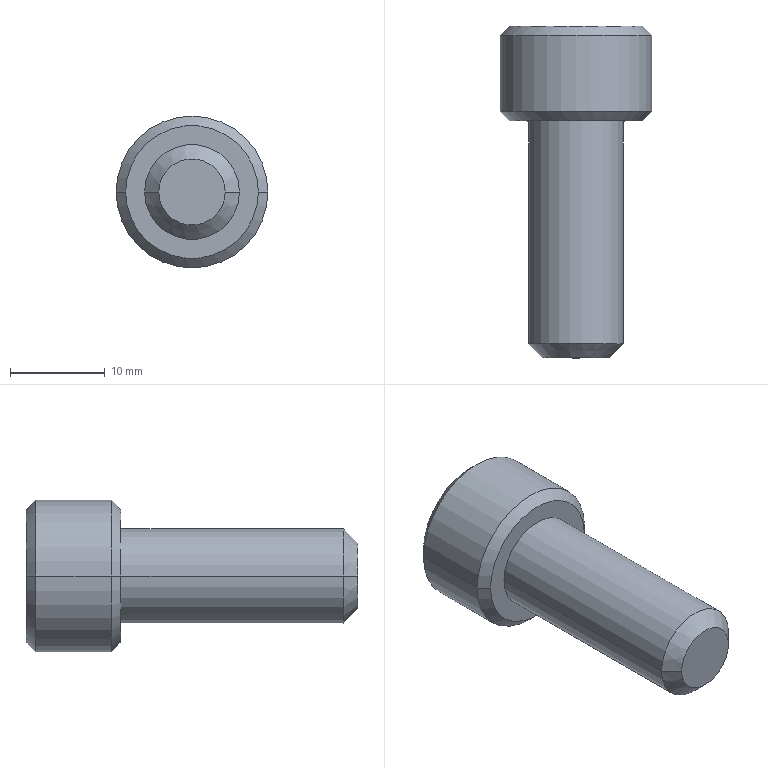Part | STEP file | BB62-M10-25L-1 | 1 solid | 27 faces | box 16 x 35 x 16 mm | volume 3564 mm3 | plane 15 | cone 8 | cylinder 4 | commonest cylinder face diameters 10 x2 16 x2
STEP:
#1=CARTESIAN_POINT('',(0.,2.359,0.));
#2=VERTEX_POINT('',#1);
#3=CARTESIAN_POINT('',(4.575,5.,0.));
#4=VERTEX_POINT('',#3);
#5=CARTESIAN_POINT('',(0.,2.359,0.));
#6=DIRECTION('',(0.866,0.5,0.));
#7=VECTOR('',#6,1000.);
#8=LINE('',#5,#7);
#9=EDGE_CURVE('',#2,#4,#8,.T.);
#10=ORIENTED_EDGE('',*,*,#9,.F.);
#11=CARTESIAN_POINT('',(-4.575,5.,0.));
#12=VERTEX_POINT('',#11);
#13=CARTESIAN_POINT('',(0.,2.359,0.));
#14=DIRECTION('',(-0.866,0.5,0.));
#15=VECTOR('',#14,1000.);
#16=LINE('',#13,#15);
#17=EDGE_CURVE('',#2,#12,#16,.T.);
#18=ORIENTED_EDGE('',*,*,#17,.T.);
#19=CARTESIAN_POINT('',(-3.962,5.,2.288));
#20=VERTEX_POINT('',#19);
#21=CARTESIAN_POINT('',(0.,5.,0.));
#22=DIRECTION('',(0.,-1.,0.));
#23=DIRECTION('',(-1.,0.,0.));
#24=AXIS2_PLACEMENT_3D('',#21,#22,#23);
#25=CIRCLE('',#24,4.575);
#26=EDGE_CURVE('',#20,#12,#25,.T.);
#27=ORIENTED_EDGE('',*,*,#26,.F.);
#28=CARTESIAN_POINT('',(0.,5.,4.575));
#29=VERTEX_POINT('',#28);
#30=CARTESIAN_POINT('',(0.,5.,0.));
#31=DIRECTION('',(0.,-1.,0.));
#32=DIRECTION('',(-1.,0.,0.));
#33=AXIS2_PLACEMENT_3D('',#30,#31,#32);
#34=CIRCLE('',#33,4.575);
#35=EDGE_CURVE('',#29,#20,#34,.T.);
#36=ORIENTED_EDGE('',*,*,#35,.F.);
#37=CARTESIAN_POINT('',(3.962,5.,2.287));
#38=VERTEX_POINT('',#37);
#39=CARTESIAN_POINT('',(0.,5.,0.));
#40=DIRECTION('',(0.,-1.,0.));
#41=DIRECTION('',(-1.,0.,0.));
#42=AXIS2_PLACEMENT_3D('',#39,#40,#41);
#43=CIRCLE('',#42,4.575);
#44=EDGE_CURVE('',#38,#29,#43,.T.);
#45=ORIENTED_EDGE('',*,*,#44,.F.);
#46=CARTESIAN_POINT('',(0.,5.,0.));
#47=DIRECTION('',(0.,-1.,0.));
#48=DIRECTION('',(-1.,0.,0.));
#49=AXIS2_PLACEMENT_3D('',#46,#47,#48);
#50=CIRCLE('',#49,4.575);
#51=EDGE_CURVE('',#4,#38,#50,.T.);
#52=ORIENTED_EDGE('',*,*,#51,.F.);
#53=EDGE_LOOP('',(#10,#18,#27,#36,#45,#52));
#54=FACE_OUTER_BOUND('',#53,.T.);
#55=CARTESIAN_POINT('',(0.,1002.359,0.));
#56=DIRECTION('',(0.,1.,0.));
#57=DIRECTION('',(1.,0.,0.));
#58=AXIS2_PLACEMENT_3D('',#55,#56,#57);
#59=CONICAL_SURFACE('',#58,1732.051,1.047);
#60=ADVANCED_FACE('',(#54),#59,.F.);
#61=CARTESIAN_POINT('',(3.5,-25.,0.));
#62=VERTEX_POINT('',#61);
#63=CARTESIAN_POINT('',(-3.5,-25.,0.));
#64=VERTEX_POINT('',#63);
#65=CARTESIAN_POINT('',(0.,-25.,0.));
#66=DIRECTION('',(0.,1.,0.));
#67=DIRECTION('',(1.,0.,0.));
#68=AXIS2_PLACEMENT_3D('',#65,#66,#67);
#69=CIRCLE('',#68,3.5);
#70=EDGE_CURVE('',#62,#64,#69,.T.);
#71=ORIENTED_EDGE('',*,*,#70,.T.);
#72=CARTESIAN_POINT('',(-5.,-23.5,0.));
#73=VERTEX_POINT('',#72);
#74=CARTESIAN_POINT('',(-3.5,-25.,0.));
#75=DIRECTION('',(-0.7071,0.7071,0.));
#76=VECTOR('',#75,1000.);
#77=LINE('',#74,#76);
#78=EDGE_CURVE('',#64,#73,#77,.T.);
#79=ORIENTED_EDGE('',*,*,#78,.T.);
#80=CARTESIAN_POINT('',(5.,-23.5,0.));
#81=VERTEX_POINT('',#80);
#82=CARTESIAN_POINT('',(0.,-23.5,0.));
#83=DIRECTION('',(0.,-1.,0.));
#84=DIRECTION('',(-1.,0.,0.));
#85=AXIS2_PLACEMENT_3D('',#82,#83,#84);
#86=CIRCLE('',#85,5.);
#87=EDGE_CURVE('',#73,#81,#86,.T.);
#88=ORIENTED_EDGE('',*,*,#87,.T.);
#89=CARTESIAN_POINT('',(3.5,-25.,0.));
#90=DIRECTION('',(0.7071,0.7071,0.));
#91=VECTOR('',#90,1000.);
#92=LINE('',#89,#91);
#93=EDGE_CURVE('',#62,#81,#92,.T.);
#94=ORIENTED_EDGE('',*,*,#93,.F.);
#95=EDGE_LOOP('',(#71,#79,#88,#94));
#96=FACE_OUTER_BOUND('',#95,.T.);
#97=CARTESIAN_POINT('',(0.,-25.,0.));
#98=DIRECTION('',(0.,1.,0.));
#99=DIRECTION('',(1.,0.,0.));
#100=AXIS2_PLACEMENT_3D('',#97,#98,#99);
#101=CONICAL_SURFACE('',#100,3.5,0.7854);
#102=ADVANCED_FACE('',(#96),#101,.T.);
#103=ORIENTED_EDGE('',*,*,#87,.F.);
#104=CARTESIAN_POINT('',(-5.,0.,0.));
#105=VERTEX_POINT('',#104);
#106=CARTESIAN_POINT('',(-5.,-23.5,0.));
#107=DIRECTION('',(0.,1.,0.));
#108=VECTOR('',#107,1000.);
#109=LINE('',#106,#108);
#110=EDGE_CURVE('',#73,#105,#109,.T.);
#111=ORIENTED_EDGE('',*,*,#110,.T.);
#112=CARTESIAN_POINT('',(5.,0.,0.));
#113=VERTEX_POINT('',#112);
#114=CARTESIAN_POINT('',(0.,0.,0.));
#115=DIRECTION('',(0.,-1.,0.));
#116=DIRECTION('',(-1.,0.,0.));
#117=AXIS2_PLACEMENT_3D('',#114,#115,#116);
#118=CIRCLE('',#117,5.);
#119=EDGE_CURVE('',#105,#113,#118,.T.);
#120=ORIENTED_EDGE('',*,*,#119,.T.);
#121=CARTESIAN_POINT('',(5.,-23.5,0.));
#122=DIRECTION('',(0.,1.,0.));
#123=VECTOR('',#122,1000.);
#124=LINE('',#121,#123);
#125=EDGE_CURVE('',#81,#113,#124,.T.);
#126=ORIENTED_EDGE('',*,*,#125,.F.);
#127=EDGE_LOOP('',(#103,#111,#120,#126));
#128=FACE_OUTER_BOUND('',#127,.T.);
#129=CARTESIAN_POINT('',(0.,-23.5,0.));
#130=DIRECTION('',(0.,1.,0.));
#131=DIRECTION('',(1.,0.,0.));
#132=AXIS2_PLACEMENT_3D('',#129,#130,#131);
#133=CYLINDRICAL_SURFACE('',#132,5.);
#134=ADVANCED_FACE('',(#128),#133,.T.);
#135=CARTESIAN_POINT('',(-7.,10.,0.));
#136=VERTEX_POINT('',#135);
#137=CARTESIAN_POINT('',(7.,10.,0.));
#138=VERTEX_POINT('',#137);
#139=CARTESIAN_POINT('',(0.,10.,0.));
#140=DIRECTION('',(0.,-1.,0.));
#141=DIRECTION('',(-1.,0.,0.));
#142=AXIS2_PLACEMENT_3D('',#139,#140,#141);
#143=CIRCLE('',#142,7.);
#144=EDGE_CURVE('',#136,#138,#143,.T.);
#145=ORIENTED_EDGE('',*,*,#144,.T.);
#146=CARTESIAN_POINT('',(8.,9.,0.));
#147=VERTEX_POINT('',#146);
#148=CARTESIAN_POINT('',(8.,9.,0.));
#149=DIRECTION('',(0.7071,-0.7071,0.));
#150=VECTOR('',#149,1000.);
#151=LINE('',#148,#150);
#152=EDGE_CURVE('',#138,#147,#151,.T.);
#153=ORIENTED_EDGE('',*,*,#152,.T.);
#154=CARTESIAN_POINT('',(-8.,9.,0.));
#155=VERTEX_POINT('',#154);
#156=CARTESIAN_POINT('',(0.,9.,0.));
#157=DIRECTION('',(0.,-1.,0.));
#158=DIRECTION('',(-1.,0.,0.));
#159=AXIS2_PLACEMENT_3D('',#156,#157,#158);
#160=CIRCLE('',#159,8.);
#161=EDGE_CURVE('',#155,#147,#160,.T.);
#162=ORIENTED_EDGE('',*,*,#161,.F.);
#163=CARTESIAN_POINT('',(-8.,9.,0.));
#164=DIRECTION('',(-0.7071,-0.7071,0.));
#165=VECTOR('',#164,1000.);
#166=LINE('',#163,#165);
#167=EDGE_CURVE('',#136,#155,#166,.T.);
#168=ORIENTED_EDGE('',*,*,#167,.F.);
#169=EDGE_LOOP('',(#145,#153,#162,#168));
#170=FACE_OUTER_BOUND('',#169,.T.);
#171=CARTESIAN_POINT('',(0.,9.,0.));
#172=DIRECTION('',(0.,-1.,0.));
#173=DIRECTION('',(-1.,0.,0.));
#174=AXIS2_PLACEMENT_3D('',#171,#172,#173);
#175=CONICAL_SURFACE('',#174,8.,0.7854);
#176=ADVANCED_FACE('',(#170),#175,.T.);
#177=ORIENTED_EDGE('',*,*,#161,.T.);
#178=CARTESIAN_POINT('',(8.,1.,0.));
#179=VERTEX_POINT('',#178);
#180=CARTESIAN_POINT('',(8.,1.62,0.));
#181=DIRECTION('',(0.,-1.,0.));
#182=VECTOR('',#181,1000.);
#183=LINE('',#180,#182);
#184=EDGE_CURVE('',#147,#179,#183,.T.);
#185=ORIENTED_EDGE('',*,*,#184,.T.);
#186=CARTESIAN_POINT('',(-8.,1.,0.));
#187=VERTEX_POINT('',#186);
#188=CARTESIAN_POINT('',(0.,1.,0.));
#189=DIRECTION('',(0.,-1.,0.));
#190=DIRECTION('',(-1.,0.,0.));
#191=AXIS2_PLACEMENT_3D('',#188,#189,#190);
#192=CIRCLE('',#191,8.);
#193=EDGE_CURVE('',#187,#179,#192,.T.);
#194=ORIENTED_EDGE('',*,*,#193,.F.);
#195=CARTESIAN_POINT('',(-8.,1.62,0.));
#196=DIRECTION('',(0.,-1.,0.));
#197=VECTOR('',#196,1000.);
#198=LINE('',#195,#197);
#199=EDGE_CURVE('',#155,#187,#198,.T.);
#200=ORIENTED_EDGE('',*,*,#199,.F.);
#201=EDGE_LOOP('',(#177,#185,#194,#200));
#202=FACE_OUTER_BOUND('',#201,.T.);
#203=CARTESIAN_POINT('',(0.,1.62,0.));
#204=DIRECTION('',(0.,-1.,0.));
#205=DIRECTION('',(-1.,0.,0.));
#206=AXIS2_PLACEMENT_3D('',#203,#204,#205);
#207=CYLINDRICAL_SURFACE('',#206,8.);
#208=ADVANCED_FACE('',(#202),#207,.T.);
#209=CARTESIAN_POINT('',(-7.,0.,0.));
#210=VERTEX_POINT('',#209);
#211=CARTESIAN_POINT('',(7.,0.,0.));
#212=VERTEX_POINT('',#211);
#213=CARTESIAN_POINT('',(0.,0.,0.));
#214=DIRECTION('',(0.,-1.,0.));
#215=DIRECTION('',(-1.,0.,0.));
#216=AXIS2_PLACEMENT_3D('',#213,#214,#215);
#217=CIRCLE('',#216,7.);
#218=EDGE_CURVE('',#210,#212,#217,.T.);
#219=ORIENTED_EDGE('',*,*,#218,.F.);
#220=CARTESIAN_POINT('',(-7.,0.,0.));
#221=DIRECTION('',(-0.7071,0.7071,0.));
#222=VECTOR('',#221,1000.);
#223=LINE('',#220,#222);
#224=EDGE_CURVE('',#210,#187,#223,.T.);
#225=ORIENTED_EDGE('',*,*,#224,.T.);
#226=ORIENTED_EDGE('',*,*,#193,.T.);
#227=CARTESIAN_POINT('',(7.,0.,0.));
#228=DIRECTION('',(0.7071,0.7071,0.));
#229=VECTOR('',#228,1000.);
#230=LINE('',#227,#229);
#231=EDGE_CURVE('',#212,#179,#230,.T.);
#232=ORIENTED_EDGE('',*,*,#231,.F.);
#233=EDGE_LOOP('',(#219,#225,#226,#232));
#234=FACE_OUTER_BOUND('',#233,.T.);
#235=CARTESIAN_POINT('',(0.,0.,0.));
#236=DIRECTION('',(0.,1.,0.));
#237=DIRECTION('',(1.,0.,0.));
#238=AXIS2_PLACEMENT_3D('',#235,#236,#237);
#239=CONICAL_SURFACE('',#238,7.,0.7854);
#240=ADVANCED_FACE('',(#234),#239,.T.);
#241=ORIENTED_EDGE('',*,*,#144,.F.);
#242=CARTESIAN_POINT('',(0.,10.,0.));
#243=DIRECTION('',(0.,-1.,0.));
#244=DIRECTION('',(-1.,0.,0.));
#245=AXIS2_PLACEMENT_3D('',#242,#243,#244);
#246=CIRCLE('',#245,7.);
#247=EDGE_CURVE('',#138,#136,#246,.T.);
#248=ORIENTED_EDGE('',*,*,#247,.F.);
#249=EDGE_LOOP('',(#241,#248));
#250=FACE_OUTER_BOUND('',#249,.T.);
#251=CARTESIAN_POINT('',(0.,10.,-4.575));
#252=VERTEX_POINT('',#251);
#253=CARTESIAN_POINT('',(-3.962,10.,-2.288));
#254=VERTEX_POINT('',#253);
#255=CARTESIAN_POINT('',(0.,10.,-4.575));
#256=DIRECTION('',(-0.866,0.,0.5));
#257=VECTOR('',#256,1000.);
#258=LINE('',#255,#257);
#259=EDGE_CURVE('',#252,#254,#258,.T.);
#260=ORIENTED_EDGE('',*,*,#259,.F.);
#261=CARTESIAN_POINT('',(3.962,10.,-2.288));
#262=VERTEX_POINT('',#261);
#263=CARTESIAN_POINT('',(3.962,10.,-2.288));
#264=DIRECTION('',(-0.866,0.,-0.5));
#265=VECTOR('',#264,1000.);
#266=LINE('',#263,#265);
#267=EDGE_CURVE('',#262,#252,#266,.T.);
#268=ORIENTED_EDGE('',*,*,#267,.F.);
#269=CARTESIAN_POINT('',(3.962,10.,2.287));
#270=VERTEX_POINT('',#269);
#271=CARTESIAN_POINT('',(3.962,10.,2.287));
#272=DIRECTION('',(0.,0.,-1.));
#273=VECTOR('',#272,1000.);
#274=LINE('',#271,#273);
#275=EDGE_CURVE('',#270,#262,#274,.T.);
#276=ORIENTED_EDGE('',*,*,#275,.F.);
#277=CARTESIAN_POINT('',(0.,10.,4.575));
#278=VERTEX_POINT('',#277);
#279=CARTESIAN_POINT('',(0.,10.,4.575));
#280=DIRECTION('',(0.866,0.,-0.5));
#281=VECTOR('',#280,1000.);
#282=LINE('',#279,#281);
#283=EDGE_CURVE('',#278,#270,#282,.T.);
#284=ORIENTED_EDGE('',*,*,#283,.F.);
#285=CARTESIAN_POINT('',(-3.962,10.,2.287));
#286=VERTEX_POINT('',#285);
#287=CARTESIAN_POINT('',(-3.962,10.,2.287));
#288=DIRECTION('',(0.866,0.,0.5));
#289=VECTOR('',#288,1000.);
#290=LINE('',#287,#289);
#291=EDGE_CURVE('',#286,#278,#290,.T.);
#292=ORIENTED_EDGE('',*,*,#291,.F.);
#293=CARTESIAN_POINT('',(-3.962,10.,-2.288));
#294=DIRECTION('',(0.,0.,1.));
#295=VECTOR('',#294,1000.);
#296=LINE('',#293,#295);
#297=EDGE_CURVE('',#254,#286,#296,.T.);
#298=ORIENTED_EDGE('',*,*,#297,.F.);
#299=EDGE_LOOP('',(#260,#268,#276,#284,#292,#298));
#300=FACE_BOUND('',#299,.T.);
#301=CARTESIAN_POINT('',(7.,10.,0.));
#302=DIRECTION('',(0.,1.,0.));
#303=DIRECTION('',(1.,0.,0.));
#304=AXIS2_PLACEMENT_3D('',#301,#302,#303);
#305=PLANE('',#304);
#306=ADVANCED_FACE('',(#250,#300),#305,.T.);
#307=CARTESIAN_POINT('',(0.,0.,0.));
#308=DIRECTION('',(0.,-1.,0.));
#309=DIRECTION('',(-1.,0.,0.));
#310=AXIS2_PLACEMENT_3D('',#307,#308,#309);
#311=CIRCLE('',#310,5.);
#312=EDGE_CURVE('',#113,#105,#311,.T.);
#313=ORIENTED_EDGE('',*,*,#312,.F.);
#314=ORIENTED_EDGE('',*,*,#119,.F.);
#315=EDGE_LOOP('',(#313,#314));
#316=FACE_BOUND('',#315,.T.);
#317=CARTESIAN_POINT('',(0.,0.,0.));
#318=DIRECTION('',(0.,-1.,0.));
#319=DIRECTION('',(-1.,0.,0.));
#320=AXIS2_PLACEMENT_3D('',#317,#318,#319);
#321=CIRCLE('',#320,7.);
#322=EDGE_CURVE('',#212,#210,#321,.T.);
#323=ORIENTED_EDGE('',*,*,#322,.T.);
#324=ORIENTED_EDGE('',*,*,#218,.T.);
#325=EDGE_LOOP('',(#323,#324));
#326=FACE_OUTER_BOUND('',#325,.T.);
#327=CARTESIAN_POINT('',(0.,0.,0.));
#328=DIRECTION('',(0.,-1.,0.));
#329=DIRECTION('',(-1.,0.,0.));
#330=AXIS2_PLACEMENT_3D('',#327,#328,#329);
#331=PLANE('',#330);
#332=ADVANCED_FACE('',(#316,#326),#331,.T.);
#333=ORIENTED_EDGE('',*,*,#224,.F.);
#334=ORIENTED_EDGE('',*,*,#322,.F.);
#335=ORIENTED_EDGE('',*,*,#231,.T.);
#336=CARTESIAN_POINT('',(0.,1.,0.));
#337=DIRECTION('',(0.,-1.,0.));
#338=DIRECTION('',(-1.,0.,0.));
#339=AXIS2_PLACEMENT_3D('',#336,#337,#338);
#340=CIRCLE('',#339,8.);
#341=EDGE_CURVE('',#179,#187,#340,.T.);
#342=ORIENTED_EDGE('',*,*,#341,.T.);
#343=EDGE_LOOP('',(#333,#334,#335,#342));
#344=FACE_OUTER_BOUND('',#343,.T.);
#345=CARTESIAN_POINT('',(0.,0.,0.));
#346=DIRECTION('',(0.,1.,0.));
#347=DIRECTION('',(1.,0.,0.));
#348=AXIS2_PLACEMENT_3D('',#345,#346,#347);
#349=CONICAL_SURFACE('',#348,7.,0.7854);
#350=ADVANCED_FACE('',(#344),#349,.T.);
#351=ORIENTED_EDGE('',*,*,#184,.F.);
#352=CARTESIAN_POINT('',(0.,9.,0.));
#353=DIRECTION('',(0.,-1.,0.));
#354=DIRECTION('',(-1.,0.,0.));
#355=AXIS2_PLACEMENT_3D('',#352,#353,#354);
#356=CIRCLE('',#355,8.);
#357=EDGE_CURVE('',#147,#155,#356,.T.);
#358=ORIENTED_EDGE('',*,*,#357,.T.);
#359=ORIENTED_EDGE('',*,*,#199,.T.);
#360=ORIENTED_EDGE('',*,*,#341,.F.);
#361=EDGE_LOOP('',(#351,#358,#359,#360));
#362=FACE_OUTER_BOUND('',#361,.T.);
#363=CARTESIAN_POINT('',(0.,1.62,0.));
#364=DIRECTION('',(0.,-1.,0.));
#365=DIRECTION('',(-1.,0.,0.));
#366=AXIS2_PLACEMENT_3D('',#363,#364,#365);
#367=CYLINDRICAL_SURFACE('',#366,8.);
#368=ADVANCED_FACE('',(#362),#367,.T.);
#369=ORIENTED_EDGE('',*,*,#152,.F.);
#370=ORIENTED_EDGE('',*,*,#247,.T.);
#371=ORIENTED_EDGE('',*,*,#167,.T.);
#372=ORIENTED_EDGE('',*,*,#357,.F.);
#373=EDGE_LOOP('',(#369,#370,#371,#372));
#374=FACE_OUTER_BOUND('',#373,.T.);
#375=CARTESIAN_POINT('',(0.,9.,0.));
#376=DIRECTION('',(0.,-1.,0.));
#377=DIRECTION('',(-1.,0.,0.));
#378=AXIS2_PLACEMENT_3D('',#375,#376,#377);
#379=CONICAL_SURFACE('',#378,8.,0.7854);
#380=ADVANCED_FACE('',(#374),#379,.T.);
#381=ORIENTED_EDGE('',*,*,#110,.F.);
#382=CARTESIAN_POINT('',(0.,-23.5,0.));
#383=DIRECTION('',(0.,-1.,0.));
#384=DIRECTION('',(-1.,0.,0.));
#385=AXIS2_PLACEMENT_3D('',#382,#383,#384);
#386=CIRCLE('',#385,5.);
#387=EDGE_CURVE('',#81,#73,#386,.T.);
#388=ORIENTED_EDGE('',*,*,#387,.F.);
#389=ORIENTED_EDGE('',*,*,#125,.T.);
#390=ORIENTED_EDGE('',*,*,#312,.T.);
#391=EDGE_LOOP('',(#381,#388,#389,#390));
#392=FACE_OUTER_BOUND('',#391,.T.);
#393=CARTESIAN_POINT('',(0.,-23.5,0.));
#394=DIRECTION('',(0.,1.,0.));
#395=DIRECTION('',(1.,0.,0.));
#396=AXIS2_PLACEMENT_3D('',#393,#394,#395);
#397=CYLINDRICAL_SURFACE('',#396,5.);
#398=ADVANCED_FACE('',(#392),#397,.T.);
#399=ORIENTED_EDGE('',*,*,#70,.F.);
#400=CARTESIAN_POINT('',(0.,-25.,0.));
#401=DIRECTION('',(0.,1.,0.));
#402=DIRECTION('',(1.,0.,0.));
#403=AXIS2_PLACEMENT_3D('',#400,#401,#402);
#404=CIRCLE('',#403,3.5);
#405=EDGE_CURVE('',#64,#62,#404,.T.);
#406=ORIENTED_EDGE('',*,*,#405,.F.);
#407=EDGE_LOOP('',(#399,#406));
#408=FACE_OUTER_BOUND('',#407,.T.);
#409=CARTESIAN_POINT('',(0.,-25.,0.));
#410=DIRECTION('',(0.,-1.,0.));
#411=DIRECTION('',(-1.,0.,0.));
#412=AXIS2_PLACEMENT_3D('',#409,#410,#411);
#413=PLANE('',#412);
#414=ADVANCED_FACE('',(#408),#413,.T.);
#415=ORIENTED_EDGE('',*,*,#78,.F.);
#416=ORIENTED_EDGE('',*,*,#405,.T.);
#417=ORIENTED_EDGE('',*,*,#93,.T.);
#418=ORIENTED_EDGE('',*,*,#387,.T.);
#419=EDGE_LOOP('',(#415,#416,#417,#418));
#420=FACE_OUTER_BOUND('',#419,.T.);
#421=CARTESIAN_POINT('',(0.,-25.,0.));
#422=DIRECTION('',(0.,1.,0.));
#423=DIRECTION('',(1.,0.,0.));
#424=AXIS2_PLACEMENT_3D('',#421,#422,#423);
#425=CONICAL_SURFACE('',#424,3.5,0.7854);
#426=ADVANCED_FACE('',(#420),#425,.T.);
#427=CARTESIAN_POINT('',(3.962,5.,-2.288));
#428=VERTEX_POINT('',#427);
#429=CARTESIAN_POINT('',(0.,5.,-4.575));
#430=VERTEX_POINT('',#429);
#431=CARTESIAN_POINT('',(3.962,5.,-2.288));
#432=DIRECTION('',(-0.866,0.,-0.5));
#433=VECTOR('',#432,1000.);
#434=LINE('',#431,#433);
#435=EDGE_CURVE('',#428,#430,#434,.T.);
#436=ORIENTED_EDGE('',*,*,#435,.F.);
#437=CARTESIAN_POINT('',(3.962,10.,-2.288));
#438=DIRECTION('',(0.,-1.,0.));
#439=VECTOR('',#438,1000.);
#440=LINE('',#437,#439);
#441=EDGE_CURVE('',#262,#428,#440,.T.);
#442=ORIENTED_EDGE('',*,*,#441,.F.);
#443=ORIENTED_EDGE('',*,*,#267,.T.);
#444=CARTESIAN_POINT('',(0.,10.,-4.575));
#445=DIRECTION('',(0.,-1.,0.));
#446=VECTOR('',#445,1000.);
#447=LINE('',#444,#446);
#448=EDGE_CURVE('',#252,#430,#447,.T.);
#449=ORIENTED_EDGE('',*,*,#448,.T.);
#450=EDGE_LOOP('',(#436,#442,#443,#449));
#451=FACE_OUTER_BOUND('',#450,.T.);
#452=CARTESIAN_POINT('',(3.962,10.,-2.288));
#453=DIRECTION('',(-0.5,0.,0.866));
#454=DIRECTION('',(0.866,0.,0.5));
#455=AXIS2_PLACEMENT_3D('',#452,#453,#454);
#456=PLANE('',#455);
#457=ADVANCED_FACE('',(#451),#456,.T.);
#458=CARTESIAN_POINT('',(-3.962,5.,-2.288));
#459=VERTEX_POINT('',#458);
#460=CARTESIAN_POINT('',(0.,5.,-4.575));
#461=DIRECTION('',(-0.866,0.,0.5));
#462=VECTOR('',#461,1000.);
#463=LINE('',#460,#462);
#464=EDGE_CURVE('',#430,#459,#463,.T.);
#465=ORIENTED_EDGE('',*,*,#464,.F.);
#466=ORIENTED_EDGE('',*,*,#448,.F.);
#467=ORIENTED_EDGE('',*,*,#259,.T.);
#468=CARTESIAN_POINT('',(-3.962,10.,-2.288));
#469=DIRECTION('',(0.,-1.,0.));
#470=VECTOR('',#469,1000.);
#471=LINE('',#468,#470);
#472=EDGE_CURVE('',#254,#459,#471,.T.);
#473=ORIENTED_EDGE('',*,*,#472,.T.);
#474=EDGE_LOOP('',(#465,#466,#467,#473));
#475=FACE_OUTER_BOUND('',#474,.T.);
#476=CARTESIAN_POINT('',(0.,10.,-4.575));
#477=DIRECTION('',(0.5,0.,0.866));
#478=DIRECTION('',(0.866,0.,-0.5));
#479=AXIS2_PLACEMENT_3D('',#476,#477,#478);
#480=PLANE('',#479);
#481=ADVANCED_FACE('',(#475),#480,.T.);
#482=CARTESIAN_POINT('',(-3.962,5.,-2.288));
#483=DIRECTION('',(0.,0.,1.));
#484=VECTOR('',#483,1000.);
#485=LINE('',#482,#484);
#486=EDGE_CURVE('',#459,#20,#485,.T.);
#487=ORIENTED_EDGE('',*,*,#486,.F.);
#488=ORIENTED_EDGE('',*,*,#472,.F.);
#489=ORIENTED_EDGE('',*,*,#297,.T.);
#490=CARTESIAN_POINT('',(-3.962,10.,2.287));
#491=DIRECTION('',(0.,-1.,0.));
#492=VECTOR('',#491,1000.);
#493=LINE('',#490,#492);
#494=EDGE_CURVE('',#286,#20,#493,.T.);
#495=ORIENTED_EDGE('',*,*,#494,.T.);
#496=EDGE_LOOP('',(#487,#488,#489,#495));
#497=FACE_OUTER_BOUND('',#496,.T.);
#498=CARTESIAN_POINT('',(-3.962,10.,-2.288));
#499=DIRECTION('',(1.,0.,0.));
#500=DIRECTION('',(0.,0.,-1.));
#501=AXIS2_PLACEMENT_3D('',#498,#499,#500);
#502=PLANE('',#501);
#503=ADVANCED_FACE('',(#497),#502,.T.);
#504=CARTESIAN_POINT('',(-3.962,5.,2.287));
#505=DIRECTION('',(0.866,0.,0.5));
#506=VECTOR('',#505,1000.);
#507=LINE('',#504,#506);
#508=EDGE_CURVE('',#20,#29,#507,.T.);
#509=ORIENTED_EDGE('',*,*,#508,.F.);
#510=ORIENTED_EDGE('',*,*,#494,.F.);
#511=ORIENTED_EDGE('',*,*,#291,.T.);
#512=CARTESIAN_POINT('',(0.,10.,4.575));
#513=DIRECTION('',(0.,-1.,0.));
#514=VECTOR('',#513,1000.);
#515=LINE('',#512,#514);
#516=EDGE_CURVE('',#278,#29,#515,.T.);
#517=ORIENTED_EDGE('',*,*,#516,.T.);
#518=EDGE_LOOP('',(#509,#510,#511,#517));
#519=FACE_OUTER_BOUND('',#518,.T.);
#520=CARTESIAN_POINT('',(-3.962,10.,2.287));
#521=DIRECTION('',(0.5,0.,-0.866));
#522=DIRECTION('',(-0.866,0.,-0.5));
#523=AXIS2_PLACEMENT_3D('',#520,#521,#522);
#524=PLANE('',#523);
#525=ADVANCED_FACE('',(#519),#524,.T.);
#526=CARTESIAN_POINT('',(0.,5.,4.575));
#527=DIRECTION('',(0.866,0.,-0.5));
#528=VECTOR('',#527,1000.);
#529=LINE('',#526,#528);
#530=EDGE_CURVE('',#29,#38,#529,.T.);
#531=ORIENTED_EDGE('',*,*,#530,.F.);
#532=ORIENTED_EDGE('',*,*,#516,.F.);
#533=ORIENTED_EDGE('',*,*,#283,.T.);
#534=CARTESIAN_POINT('',(3.962,10.,2.287));
#535=DIRECTION('',(0.,-1.,0.));
#536=VECTOR('',#535,1000.);
#537=LINE('',#534,#536);
#538=EDGE_CURVE('',#270,#38,#537,.T.);
#539=ORIENTED_EDGE('',*,*,#538,.T.);
#540=EDGE_LOOP('',(#531,#532,#533,#539));
#541=FACE_OUTER_BOUND('',#540,.T.);
#542=CARTESIAN_POINT('',(0.,10.,4.575));
#543=DIRECTION('',(-0.5,0.,-0.866));
#544=DIRECTION('',(-0.866,0.,0.5));
#545=AXIS2_PLACEMENT_3D('',#542,#543,#544);
#546=PLANE('',#545);
#547=ADVANCED_FACE('',(#541),#546,.T.);
#548=CARTESIAN_POINT('',(3.962,5.,2.287));
#549=DIRECTION('',(0.,0.,-1.));
#550=VECTOR('',#549,1000.);
#551=LINE('',#548,#550);
#552=EDGE_CURVE('',#38,#428,#551,.T.);
#553=ORIENTED_EDGE('',*,*,#552,.F.);
#554=ORIENTED_EDGE('',*,*,#538,.F.);
#555=ORIENTED_EDGE('',*,*,#275,.T.);
#556=ORIENTED_EDGE('',*,*,#441,.T.);
#557=EDGE_LOOP('',(#553,#554,#555,#556));
#558=FACE_OUTER_BOUND('',#557,.T.);
#559=CARTESIAN_POINT('',(3.962,10.,2.287));
#560=DIRECTION('',(-1.,0.,0.));
#561=DIRECTION('',(0.,0.,1.));
#562=AXIS2_PLACEMENT_3D('',#559,#560,#561);
#563=PLANE('',#562);
#564=ADVANCED_FACE('',(#558),#563,.T.);
#565=ORIENTED_EDGE('',*,*,#435,.T.);
#566=CARTESIAN_POINT('',(0.,5.,0.));
#567=DIRECTION('',(0.,-1.,0.));
#568=DIRECTION('',(-1.,0.,0.));
#569=AXIS2_PLACEMENT_3D('',#566,#567,#568);
#570=CIRCLE('',#569,4.575);
#571=EDGE_CURVE('',#430,#428,#570,.T.);
#572=ORIENTED_EDGE('',*,*,#571,.T.);
#573=EDGE_LOOP('',(#565,#572));
#574=FACE_OUTER_BOUND('',#573,.T.);
#575=CARTESIAN_POINT('',(0.,5.,0.));
#576=DIRECTION('',(0.,1.,0.));
#577=DIRECTION('',(1.,0.,0.));
#578=AXIS2_PLACEMENT_3D('',#575,#576,#577);
#579=PLANE('',#578);
#580=ADVANCED_FACE('',(#574),#579,.F.);
#581=ORIENTED_EDGE('',*,*,#552,.T.);
#582=CARTESIAN_POINT('',(0.,5.,0.));
#583=DIRECTION('',(0.,-1.,0.));
#584=DIRECTION('',(-1.,0.,0.));
#585=AXIS2_PLACEMENT_3D('',#582,#583,#584);
#586=CIRCLE('',#585,4.575);
#587=EDGE_CURVE('',#428,#4,#586,.T.);
#588=ORIENTED_EDGE('',*,*,#587,.T.);
#589=ORIENTED_EDGE('',*,*,#51,.T.);
#590=EDGE_LOOP('',(#581,#588,#589));
#591=FACE_OUTER_BOUND('',#590,.T.);
#592=CARTESIAN_POINT('',(0.,5.,0.));
#593=DIRECTION('',(0.,1.,0.));
#594=DIRECTION('',(1.,0.,0.));
#595=AXIS2_PLACEMENT_3D('',#592,#593,#594);
#596=PLANE('',#595);
#597=ADVANCED_FACE('',(#591),#596,.F.);
#598=ORIENTED_EDGE('',*,*,#530,.T.);
#599=ORIENTED_EDGE('',*,*,#44,.T.);
#600=EDGE_LOOP('',(#598,#599));
#601=FACE_OUTER_BOUND('',#600,.T.);
#602=CARTESIAN_POINT('',(0.,5.,0.));
#603=DIRECTION('',(0.,1.,0.));
#604=DIRECTION('',(1.,0.,0.));
#605=AXIS2_PLACEMENT_3D('',#602,#603,#604);
#606=PLANE('',#605);
#607=ADVANCED_FACE('',(#601),#606,.F.);
#608=ORIENTED_EDGE('',*,*,#508,.T.);
#609=ORIENTED_EDGE('',*,*,#35,.T.);
#610=EDGE_LOOP('',(#608,#609));
#611=FACE_OUTER_BOUND('',#610,.T.);
#612=CARTESIAN_POINT('',(0.,5.,0.));
#613=DIRECTION('',(0.,1.,0.));
#614=DIRECTION('',(1.,0.,0.));
#615=AXIS2_PLACEMENT_3D('',#612,#613,#614);
#616=PLANE('',#615);
#617=ADVANCED_FACE('',(#611),#616,.F.);
#618=ORIENTED_EDGE('',*,*,#486,.T.);
#619=ORIENTED_EDGE('',*,*,#26,.T.);
#620=CARTESIAN_POINT('',(0.,5.,0.));
#621=DIRECTION('',(0.,-1.,0.));
#622=DIRECTION('',(-1.,0.,0.));
#623=AXIS2_PLACEMENT_3D('',#620,#621,#622);
#624=CIRCLE('',#623,4.575);
#625=EDGE_CURVE('',#12,#459,#624,.T.);
#626=ORIENTED_EDGE('',*,*,#625,.T.);
#627=EDGE_LOOP('',(#618,#619,#626));
#628=FACE_OUTER_BOUND('',#627,.T.);
#629=CARTESIAN_POINT('',(0.,5.,0.));
#630=DIRECTION('',(0.,1.,0.));
#631=DIRECTION('',(1.,0.,0.));
#632=AXIS2_PLACEMENT_3D('',#629,#630,#631);
#633=PLANE('',#632);
#634=ADVANCED_FACE('',(#628),#633,.F.);
#635=ORIENTED_EDGE('',*,*,#464,.T.);
#636=CARTESIAN_POINT('',(0.,5.,0.));
#637=DIRECTION('',(0.,-1.,0.));
#638=DIRECTION('',(-1.,0.,0.));
#639=AXIS2_PLACEMENT_3D('',#636,#637,#638);
#640=CIRCLE('',#639,4.575);
#641=EDGE_CURVE('',#459,#430,#640,.T.);
#642=ORIENTED_EDGE('',*,*,#641,.T.);
#643=EDGE_LOOP('',(#635,#642));
#644=FACE_OUTER_BOUND('',#643,.T.);
#645=CARTESIAN_POINT('',(0.,5.,0.));
#646=DIRECTION('',(0.,1.,0.));
#647=DIRECTION('',(1.,0.,0.));
#648=AXIS2_PLACEMENT_3D('',#645,#646,#647);
#649=PLANE('',#648);
#650=ADVANCED_FACE('',(#644),#649,.F.);
#651=ORIENTED_EDGE('',*,*,#17,.F.);
#652=ORIENTED_EDGE('',*,*,#9,.T.);
#653=ORIENTED_EDGE('',*,*,#587,.F.);
#654=ORIENTED_EDGE('',*,*,#571,.F.);
#655=ORIENTED_EDGE('',*,*,#641,.F.);
#656=ORIENTED_EDGE('',*,*,#625,.F.);
#657=EDGE_LOOP('',(#651,#652,#653,#654,#655,#656));
#658=FACE_OUTER_BOUND('',#657,.T.);
#659=CARTESIAN_POINT('',(0.,1002.359,0.));
#660=DIRECTION('',(0.,1.,0.));
#661=DIRECTION('',(1.,0.,0.));
#662=AXIS2_PLACEMENT_3D('',#659,#660,#661);
#663=CONICAL_SURFACE('',#662,1732.051,1.047);
#664=ADVANCED_FACE('',(#658),#663,.F.);
#665=CLOSED_SHELL('',(#60,#102,#134,#176,#208,#240,#306,#332,#350,#368,#380,#398,#414,#426,#457,#481,#503,#525,#547,#564,#580,#597,#607,#617,#634,#650,#664));
#666=MANIFOLD_SOLID_BREP('',#665);
#667=CARTESIAN_POINT('',(0.,0.,0.));
#668=DIRECTION('',(0.,0.,1.));
#669=DIRECTION('',(1.,0.,0.));
#670=AXIS2_PLACEMENT_3D('',#667,#668,#669);
#671=(LENGTH_UNIT()NAMED_UNIT(*)SI_UNIT(.MILLI.,.METRE.));
#672=UNCERTAINTY_MEASURE_WITH_UNIT(LENGTH_MEASURE(0.00001),#671,'','');
#673=(NAMED_UNIT(*)PLANE_ANGLE_UNIT()SI_UNIT($,.RADIAN.));
#674=(NAMED_UNIT(*)SI_UNIT($,.STERADIAN.)SOLID_ANGLE_UNIT());
#675=(GEOMETRIC_REPRESENTATION_CONTEXT(3)GLOBAL_UNCERTAINTY_ASSIGNED_CONTEXT((#672))GLOBAL_UNIT_ASSIGNED_CONTEXT((#671,#673,#674))REPRESENTATION_CONTEXT('',''));
#676=ADVANCED_BREP_SHAPE_REPRESENTATION('',(#666,#670),#675);